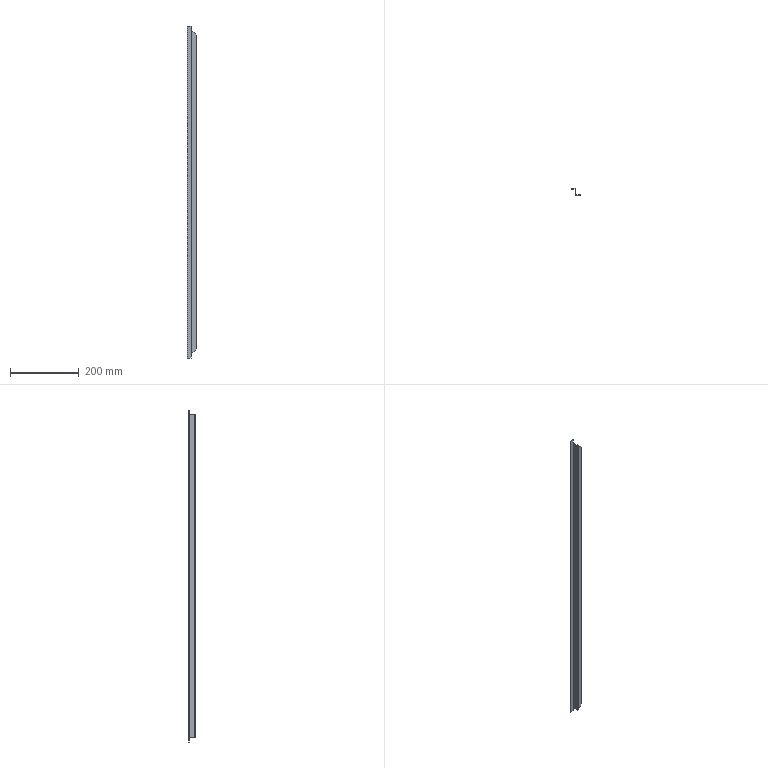Part | STEP file | Left Side Panel Frame Upper | 1 solid | 28 faces | box 26.5 x 20 x 964 mm | volume 62237 mm3 | plane 22 | cylinder 6 | commonest cylinder face diameters 0.15 x2 0.2 x1 1 x1 3.2 x1 4 x1
STEP:
#1=CARTESIAN_POINT('',(0.,-25.93,127.648));
#2=VERTEX_POINT('',#1);
#3=CARTESIAN_POINT('',(0.,-28.08,127.648));
#4=VERTEX_POINT('',#3);
#5=CARTESIAN_POINT('',(0.,0.,127.648));
#6=DIRECTION('',(0.,-1.,0.));
#7=VECTOR('',#6,1000.);
#8=LINE('',#5,#7);
#9=EDGE_CURVE('',#2,#4,#8,.T.);
#10=ORIENTED_EDGE('',*,*,#9,.T.);
#11=CARTESIAN_POINT('',(0.,-28.08,127.598));
#12=VERTEX_POINT('',#11);
#13=CARTESIAN_POINT('',(0.,-28.08,1067.598));
#14=DIRECTION('',(0.,0.,1.));
#15=VECTOR('',#14,1000.);
#16=LINE('',#13,#15);
#17=EDGE_CURVE('',#12,#4,#16,.T.);
#18=ORIENTED_EDGE('',*,*,#17,.F.);
#19=CARTESIAN_POINT('',(0.,-9.68,127.598));
#20=VERTEX_POINT('',#19);
#21=CARTESIAN_POINT('',(0.,0.,127.598));
#22=DIRECTION('',(0.,1.,0.));
#23=VECTOR('',#22,1000.);
#24=LINE('',#21,#23);
#25=EDGE_CURVE('',#12,#20,#24,.T.);
#26=ORIENTED_EDGE('',*,*,#25,.T.);
#27=CARTESIAN_POINT('',(0.,-9.68,1067.598));
#28=VERTEX_POINT('',#27);
#29=CARTESIAN_POINT('',(0.,-9.68,0.));
#30=DIRECTION('',(0.,0.,1.));
#31=VECTOR('',#30,1000.);
#32=LINE('',#29,#31);
#33=EDGE_CURVE('',#20,#28,#32,.T.);
#34=ORIENTED_EDGE('',*,*,#33,.T.);
#35=CARTESIAN_POINT('',(0.,-28.08,1067.598));
#36=VERTEX_POINT('',#35);
#37=CARTESIAN_POINT('',(0.,0.,1067.598));
#38=DIRECTION('',(0.,-1.,0.));
#39=VECTOR('',#38,1000.);
#40=LINE('',#37,#39);
#41=EDGE_CURVE('',#28,#36,#40,.T.);
#42=ORIENTED_EDGE('',*,*,#41,.T.);
#43=CARTESIAN_POINT('',(0.,-28.08,1067.548));
#44=VERTEX_POINT('',#43);
#45=CARTESIAN_POINT('',(0.,-28.08,1067.598));
#46=DIRECTION('',(0.,0.,1.));
#47=VECTOR('',#46,1000.);
#48=LINE('',#45,#47);
#49=EDGE_CURVE('',#44,#36,#48,.T.);
#50=ORIENTED_EDGE('',*,*,#49,.F.);
#51=CARTESIAN_POINT('',(0.,-25.93,1067.548));
#52=VERTEX_POINT('',#51);
#53=CARTESIAN_POINT('',(0.,0.,1067.548));
#54=DIRECTION('',(0.,1.,0.));
#55=VECTOR('',#54,1000.);
#56=LINE('',#53,#55);
#57=EDGE_CURVE('',#44,#52,#56,.T.);
#58=ORIENTED_EDGE('',*,*,#57,.T.);
#59=CARTESIAN_POINT('',(0.,-25.93,1067.398));
#60=VERTEX_POINT('',#59);
#61=CARTESIAN_POINT('',(0.,-25.93,1067.473));
#62=DIRECTION('',(-1.,0.,0.));
#63=DIRECTION('',(0.,0.,1.));
#64=AXIS2_PLACEMENT_3D('',#61,#62,#63);
#65=CIRCLE('',#64,0.075);
#66=EDGE_CURVE('',#52,#60,#65,.T.);
#67=ORIENTED_EDGE('',*,*,#66,.T.);
#68=CARTESIAN_POINT('',(0.,-26.08,1067.398));
#69=VERTEX_POINT('',#68);
#70=CARTESIAN_POINT('',(0.,-26.08,1067.398));
#71=DIRECTION('',(0.,1.,0.));
#72=VECTOR('',#71,1000.);
#73=LINE('',#70,#72);
#74=EDGE_CURVE('',#69,#60,#73,.T.);
#75=ORIENTED_EDGE('',*,*,#74,.F.);
#76=CARTESIAN_POINT('',(0.,-26.08,127.798));
#77=VERTEX_POINT('',#76);
#78=CARTESIAN_POINT('',(0.,-26.08,0.));
#79=DIRECTION('',(0.,0.,-1.));
#80=VECTOR('',#79,1000.);
#81=LINE('',#78,#80);
#82=EDGE_CURVE('',#69,#77,#81,.T.);
#83=ORIENTED_EDGE('',*,*,#82,.T.);
#84=CARTESIAN_POINT('',(0.,-25.93,127.798));
#85=VERTEX_POINT('',#84);
#86=CARTESIAN_POINT('',(0.,-25.93,127.798));
#87=DIRECTION('',(0.,-1.,0.));
#88=VECTOR('',#87,1000.);
#89=LINE('',#86,#88);
#90=EDGE_CURVE('',#85,#77,#89,.T.);
#91=ORIENTED_EDGE('',*,*,#90,.F.);
#92=CARTESIAN_POINT('',(0.,-25.93,127.723));
#93=DIRECTION('',(-1.,0.,0.));
#94=DIRECTION('',(0.,0.,1.));
#95=AXIS2_PLACEMENT_3D('',#92,#93,#94);
#96=CIRCLE('',#95,0.075);
#97=EDGE_CURVE('',#85,#2,#96,.T.);
#98=ORIENTED_EDGE('',*,*,#97,.T.);
#99=EDGE_LOOP('',(#10,#18,#26,#34,#42,#50,#58,#67,#75,#83,#91,#98));
#100=FACE_OUTER_BOUND('',#99,.T.);
#101=CARTESIAN_POINT('',(0.,0.,0.));
#102=DIRECTION('',(1.,0.,0.));
#103=DIRECTION('',(0.,0.,-1.));
#104=AXIS2_PLACEMENT_3D('',#101,#102,#103);
#105=PLANE('',#104);
#106=ADVANCED_FACE('',(#100),#105,.T.);
#107=CARTESIAN_POINT('',(-1.5,-28.08,127.648));
#108=VERTEX_POINT('',#107);
#109=CARTESIAN_POINT('',(0.,-28.08,127.648));
#110=DIRECTION('',(1.,0.,0.));
#111=VECTOR('',#110,1000.);
#112=LINE('',#109,#111);
#113=EDGE_CURVE('',#108,#4,#112,.T.);
#114=ORIENTED_EDGE('',*,*,#113,.T.);
#115=ORIENTED_EDGE('',*,*,#9,.F.);
#116=CARTESIAN_POINT('',(-1.5,-25.93,127.648));
#117=VERTEX_POINT('',#116);
#118=CARTESIAN_POINT('',(0.,-25.93,127.648));
#119=DIRECTION('',(-1.,0.,0.));
#120=VECTOR('',#119,1000.);
#121=LINE('',#118,#120);
#122=EDGE_CURVE('',#2,#117,#121,.T.);
#123=ORIENTED_EDGE('',*,*,#122,.T.);
#124=CARTESIAN_POINT('',(-1.5,-28.08,127.648));
#125=DIRECTION('',(0.,-1.,0.));
#126=VECTOR('',#125,1000.);
#127=LINE('',#124,#126);
#128=EDGE_CURVE('',#117,#108,#127,.T.);
#129=ORIENTED_EDGE('',*,*,#128,.T.);
#130=EDGE_LOOP('',(#114,#115,#123,#129));
#131=FACE_OUTER_BOUND('',#130,.T.);
#132=CARTESIAN_POINT('',(0.,-28.08,127.648));
#133=DIRECTION('',(0.,0.,1.));
#134=DIRECTION('',(0.,-1.,0.));
#135=AXIS2_PLACEMENT_3D('',#132,#133,#134);
#136=PLANE('',#135);
#137=ADVANCED_FACE('',(#131),#136,.T.);
#138=CARTESIAN_POINT('',(0.5,-26.58,1067.098));
#139=VERTEX_POINT('',#138);
#140=CARTESIAN_POINT('',(0.2,-26.48,1067.398));
#141=VERTEX_POINT('',#140);
#142=CARTESIAN_POINT('',(0.5,-26.58,1067.098));
#143=CARTESIAN_POINT('',(0.3909,-26.58,1067.207));
#144=CARTESIAN_POINT('',(0.2873,-26.546,1067.311));
#145=CARTESIAN_POINT('',(0.2,-26.48,1067.398));
#146=(BOUNDED_CURVE()B_SPLINE_CURVE(3,(#142,#143,#144,#145),.UNSPECIFIED.,.F.,.F.)B_SPLINE_CURVE_WITH_KNOTS((4,4),(1.571,2.214),.UNSPECIFIED.)CURVE()GEOMETRIC_REPRESENTATION_ITEM()RATIONAL_B_SPLINE_CURVE((1.,0.9658,0.9658,1.))REPRESENTATION_ITEM(''));
#147=EDGE_CURVE('',#139,#141,#146,.T.);
#148=ORIENTED_EDGE('',*,*,#147,.F.);
#149=CARTESIAN_POINT('',(0.5,-26.58,128.098));
#150=VERTEX_POINT('',#149);
#151=CARTESIAN_POINT('',(0.5,-26.58,127.798));
#152=DIRECTION('',(0.,0.,1.));
#153=VECTOR('',#152,1000.);
#154=LINE('',#151,#153);
#155=EDGE_CURVE('',#150,#139,#154,.T.);
#156=ORIENTED_EDGE('',*,*,#155,.F.);
#157=CARTESIAN_POINT('',(0.2,-26.48,127.798));
#158=VERTEX_POINT('',#157);
#159=CARTESIAN_POINT('',(0.5,-26.58,128.098));
#160=CARTESIAN_POINT('',(0.3909,-26.58,127.989));
#161=CARTESIAN_POINT('',(0.2873,-26.546,127.885));
#162=CARTESIAN_POINT('',(0.2,-26.48,127.798));
#163=(BOUNDED_CURVE()B_SPLINE_CURVE(3,(#159,#160,#161,#162),.UNSPECIFIED.,.F.,.F.)B_SPLINE_CURVE_WITH_KNOTS((4,4),(4.712,5.356),.UNSPECIFIED.)CURVE()GEOMETRIC_REPRESENTATION_ITEM()RATIONAL_B_SPLINE_CURVE((1.,0.9658,0.9658,1.))REPRESENTATION_ITEM(''));
#164=EDGE_CURVE('',#150,#158,#163,.T.);
#165=ORIENTED_EDGE('',*,*,#164,.T.);
#166=CARTESIAN_POINT('',(0.5,-26.08,127.798));
#167=DIRECTION('',(0.,0.,-1.));
#168=DIRECTION('',(-1.,0.,0.));
#169=AXIS2_PLACEMENT_3D('',#166,#167,#168);
#170=CIRCLE('',#169,0.5);
#171=EDGE_CURVE('',#158,#77,#170,.T.);
#172=ORIENTED_EDGE('',*,*,#171,.T.);
#173=ORIENTED_EDGE('',*,*,#82,.F.);
#174=CARTESIAN_POINT('',(0.5,-26.08,1067.398));
#175=DIRECTION('',(0.,0.,-1.));
#176=DIRECTION('',(-1.,0.,0.));
#177=AXIS2_PLACEMENT_3D('',#174,#175,#176);
#178=CIRCLE('',#177,0.5);
#179=EDGE_CURVE('',#141,#69,#178,.T.);
#180=ORIENTED_EDGE('',*,*,#179,.F.);
#181=EDGE_LOOP('',(#148,#156,#165,#172,#173,#180));
#182=FACE_OUTER_BOUND('',#181,.T.);
#183=CARTESIAN_POINT('',(0.5,-26.08,127.798));
#184=DIRECTION('',(0.,0.,-1.));
#185=DIRECTION('',(-1.,0.,0.));
#186=AXIS2_PLACEMENT_3D('',#183,#184,#185);
#187=CYLINDRICAL_SURFACE('',#186,0.5);
#188=ADVANCED_FACE('',(#182),#187,.F.);
#189=CARTESIAN_POINT('',(-1.5,-25.93,1067.548));
#190=VERTEX_POINT('',#189);
#191=CARTESIAN_POINT('',(0.,-25.93,1067.548));
#192=DIRECTION('',(1.,0.,0.));
#193=VECTOR('',#192,1000.);
#194=LINE('',#191,#193);
#195=EDGE_CURVE('',#190,#52,#194,.T.);
#196=ORIENTED_EDGE('',*,*,#195,.T.);
#197=ORIENTED_EDGE('',*,*,#57,.F.);
#198=CARTESIAN_POINT('',(-1.5,-28.08,1067.548));
#199=VERTEX_POINT('',#198);
#200=CARTESIAN_POINT('',(0.,-28.08,1067.548));
#201=DIRECTION('',(-1.,0.,0.));
#202=VECTOR('',#201,1000.);
#203=LINE('',#200,#202);
#204=EDGE_CURVE('',#44,#199,#203,.T.);
#205=ORIENTED_EDGE('',*,*,#204,.T.);
#206=CARTESIAN_POINT('',(-1.5,-25.93,1067.548));
#207=DIRECTION('',(0.,1.,0.));
#208=VECTOR('',#207,1000.);
#209=LINE('',#206,#208);
#210=EDGE_CURVE('',#199,#190,#209,.T.);
#211=ORIENTED_EDGE('',*,*,#210,.T.);
#212=EDGE_LOOP('',(#196,#197,#205,#211));
#213=FACE_OUTER_BOUND('',#212,.T.);
#214=CARTESIAN_POINT('',(0.,-25.93,1067.548));
#215=DIRECTION('',(0.,0.,-1.));
#216=DIRECTION('',(-1.,0.,0.));
#217=AXIS2_PLACEMENT_3D('',#214,#215,#216);
#218=PLANE('',#217);
#219=ADVANCED_FACE('',(#213),#218,.T.);
#220=CARTESIAN_POINT('',(-1.5,-28.08,1067.598));
#221=VERTEX_POINT('',#220);
#222=CARTESIAN_POINT('',(-1.5,-28.08,1067.598));
#223=DIRECTION('',(1.,0.,0.));
#224=VECTOR('',#223,1000.);
#225=LINE('',#222,#224);
#226=EDGE_CURVE('',#221,#36,#225,.T.);
#227=ORIENTED_EDGE('',*,*,#226,.T.);
#228=ORIENTED_EDGE('',*,*,#41,.F.);
#229=CARTESIAN_POINT('',(-1.6,-8.08,1067.598));
#230=VERTEX_POINT('',#229);
#231=CARTESIAN_POINT('',(-1.6,-9.68,1067.598));
#232=DIRECTION('',(0.,0.,-1.));
#233=DIRECTION('',(-1.,0.,0.));
#234=AXIS2_PLACEMENT_3D('',#231,#232,#233);
#235=CIRCLE('',#234,1.6);
#236=EDGE_CURVE('',#230,#28,#235,.T.);
#237=ORIENTED_EDGE('',*,*,#236,.F.);
#238=CARTESIAN_POINT('',(-1.6,-9.58,1067.598));
#239=VERTEX_POINT('',#238);
#240=CARTESIAN_POINT('',(-1.6,-9.58,1067.598));
#241=DIRECTION('',(0.,-1.,0.));
#242=VECTOR('',#241,1000.);
#243=LINE('',#240,#242);
#244=EDGE_CURVE('',#230,#239,#243,.T.);
#245=ORIENTED_EDGE('',*,*,#244,.T.);
#246=CARTESIAN_POINT('',(-1.5,-9.68,1067.598));
#247=VERTEX_POINT('',#246);
#248=CARTESIAN_POINT('',(-1.6,-9.68,1067.598));
#249=DIRECTION('',(0.,0.,-1.));
#250=DIRECTION('',(-1.,0.,0.));
#251=AXIS2_PLACEMENT_3D('',#248,#249,#250);
#252=CIRCLE('',#251,0.1);
#253=EDGE_CURVE('',#239,#247,#252,.T.);
#254=ORIENTED_EDGE('',*,*,#253,.T.);
#255=CARTESIAN_POINT('',(-1.5,-8.08,1067.598));
#256=DIRECTION('',(0.,-1.,0.));
#257=VECTOR('',#256,1000.);
#258=LINE('',#255,#257);
#259=EDGE_CURVE('',#247,#221,#258,.T.);
#260=ORIENTED_EDGE('',*,*,#259,.T.);
#261=EDGE_LOOP('',(#227,#228,#237,#245,#254,#260));
#262=FACE_OUTER_BOUND('',#261,.T.);
#263=CARTESIAN_POINT('',(-1.5,-8.08,1067.598));
#264=DIRECTION('',(0.,0.,1.));
#265=DIRECTION('',(1.,0.,0.));
#266=AXIS2_PLACEMENT_3D('',#263,#264,#265);
#267=PLANE('',#266);
#268=ADVANCED_FACE('',(#262),#267,.T.);
#269=CARTESIAN_POINT('',(-1.6,-8.08,127.598));
#270=VERTEX_POINT('',#269);
#271=CARTESIAN_POINT('',(-1.6,-8.08,127.598));
#272=DIRECTION('',(0.,0.,1.));
#273=VECTOR('',#272,1000.);
#274=LINE('',#271,#273);
#275=EDGE_CURVE('',#270,#230,#274,.T.);
#276=ORIENTED_EDGE('',*,*,#275,.T.);
#277=ORIENTED_EDGE('',*,*,#236,.T.);
#278=ORIENTED_EDGE('',*,*,#33,.F.);
#279=CARTESIAN_POINT('',(-1.6,-9.68,127.598));
#280=DIRECTION('',(0.,0.,1.));
#281=DIRECTION('',(-1.,0.,0.));
#282=AXIS2_PLACEMENT_3D('',#279,#280,#281);
#283=CIRCLE('',#282,1.6);
#284=EDGE_CURVE('',#20,#270,#283,.T.);
#285=ORIENTED_EDGE('',*,*,#284,.T.);
#286=EDGE_LOOP('',(#276,#277,#278,#285));
#287=FACE_OUTER_BOUND('',#286,.T.);
#288=CARTESIAN_POINT('',(-1.6,-9.68,127.598));
#289=DIRECTION('',(0.,0.,-1.));
#290=DIRECTION('',(-1.,0.,0.));
#291=AXIS2_PLACEMENT_3D('',#288,#289,#290);
#292=CYLINDRICAL_SURFACE('',#291,1.6);
#293=ADVANCED_FACE('',(#287),#292,.T.);
#294=ORIENTED_EDGE('',*,*,#25,.F.);
#295=CARTESIAN_POINT('',(-1.5,-28.08,127.598));
#296=VERTEX_POINT('',#295);
#297=CARTESIAN_POINT('',(-1.5,-28.08,127.598));
#298=DIRECTION('',(-1.,0.,0.));
#299=VECTOR('',#298,1000.);
#300=LINE('',#297,#299);
#301=EDGE_CURVE('',#12,#296,#300,.T.);
#302=ORIENTED_EDGE('',*,*,#301,.T.);
#303=CARTESIAN_POINT('',(-1.5,-9.68,127.598));
#304=VERTEX_POINT('',#303);
#305=CARTESIAN_POINT('',(-1.5,-28.08,127.598));
#306=DIRECTION('',(0.,1.,0.));
#307=VECTOR('',#306,1000.);
#308=LINE('',#305,#307);
#309=EDGE_CURVE('',#296,#304,#308,.T.);
#310=ORIENTED_EDGE('',*,*,#309,.T.);
#311=CARTESIAN_POINT('',(-1.6,-9.58,127.598));
#312=VERTEX_POINT('',#311);
#313=CARTESIAN_POINT('',(-1.6,-9.68,127.598));
#314=DIRECTION('',(0.,0.,-1.));
#315=DIRECTION('',(-1.,0.,0.));
#316=AXIS2_PLACEMENT_3D('',#313,#314,#315);
#317=CIRCLE('',#316,0.1);
#318=EDGE_CURVE('',#312,#304,#317,.T.);
#319=ORIENTED_EDGE('',*,*,#318,.F.);
#320=CARTESIAN_POINT('',(-1.6,-9.68,127.598));
#321=DIRECTION('',(0.,-1.,0.));
#322=VECTOR('',#321,1000.);
#323=LINE('',#320,#322);
#324=EDGE_CURVE('',#270,#312,#323,.T.);
#325=ORIENTED_EDGE('',*,*,#324,.F.);
#326=ORIENTED_EDGE('',*,*,#284,.F.);
#327=EDGE_LOOP('',(#294,#302,#310,#319,#325,#326));
#328=FACE_OUTER_BOUND('',#327,.T.);
#329=CARTESIAN_POINT('',(-1.5,-28.08,127.598));
#330=DIRECTION('',(0.,0.,-1.));
#331=DIRECTION('',(-1.,0.,0.));
#332=AXIS2_PLACEMENT_3D('',#329,#330,#331);
#333=PLANE('',#332);
#334=ADVANCED_FACE('',(#328),#333,.T.);
#335=CARTESIAN_POINT('',(-1.5,-28.08,1067.598));
#336=DIRECTION('',(0.,0.,-1.));
#337=VECTOR('',#336,1000.);
#338=LINE('',#335,#337);
#339=EDGE_CURVE('',#108,#296,#338,.T.);
#340=ORIENTED_EDGE('',*,*,#339,.T.);
#341=ORIENTED_EDGE('',*,*,#301,.F.);
#342=ORIENTED_EDGE('',*,*,#17,.T.);
#343=ORIENTED_EDGE('',*,*,#113,.F.);
#344=EDGE_LOOP('',(#340,#341,#342,#343));
#345=FACE_OUTER_BOUND('',#344,.T.);
#346=CARTESIAN_POINT('',(-1.5,-28.08,1067.598));
#347=DIRECTION('',(0.,-1.,0.));
#348=DIRECTION('',(0.,0.,-1.));
#349=AXIS2_PLACEMENT_3D('',#346,#347,#348);
#350=PLANE('',#349);
#351=ADVANCED_FACE('',(#345),#350,.T.);
#352=ORIENTED_EDGE('',*,*,#309,.F.);
#353=ORIENTED_EDGE('',*,*,#339,.F.);
#354=ORIENTED_EDGE('',*,*,#128,.F.);
#355=CARTESIAN_POINT('',(-1.5,-25.93,127.798));
#356=VERTEX_POINT('',#355);
#357=CARTESIAN_POINT('',(-1.5,-25.93,127.723));
#358=DIRECTION('',(-1.,0.,0.));
#359=DIRECTION('',(0.,0.,1.));
#360=AXIS2_PLACEMENT_3D('',#357,#358,#359);
#361=CIRCLE('',#360,0.075);
#362=EDGE_CURVE('',#356,#117,#361,.T.);
#363=ORIENTED_EDGE('',*,*,#362,.F.);
#364=CARTESIAN_POINT('',(-1.5,-26.08,127.798));
#365=VERTEX_POINT('',#364);
#366=CARTESIAN_POINT('',(-1.5,-25.93,127.798));
#367=DIRECTION('',(0.,1.,0.));
#368=VECTOR('',#367,1000.);
#369=LINE('',#366,#368);
#370=EDGE_CURVE('',#365,#356,#369,.T.);
#371=ORIENTED_EDGE('',*,*,#370,.F.);
#372=CARTESIAN_POINT('',(-1.5,-26.08,1067.398));
#373=VERTEX_POINT('',#372);
#374=CARTESIAN_POINT('',(-1.5,-26.08,0.));
#375=DIRECTION('',(0.,0.,-1.));
#376=VECTOR('',#375,1000.);
#377=LINE('',#374,#376);
#378=EDGE_CURVE('',#373,#365,#377,.T.);
#379=ORIENTED_EDGE('',*,*,#378,.F.);
#380=CARTESIAN_POINT('',(-1.5,-25.93,1067.398));
#381=VERTEX_POINT('',#380);
#382=CARTESIAN_POINT('',(-1.5,-26.08,1067.398));
#383=DIRECTION('',(0.,-1.,0.));
#384=VECTOR('',#383,1000.);
#385=LINE('',#382,#384);
#386=EDGE_CURVE('',#381,#373,#385,.T.);
#387=ORIENTED_EDGE('',*,*,#386,.F.);
#388=CARTESIAN_POINT('',(-1.5,-25.93,1067.473));
#389=DIRECTION('',(-1.,0.,0.));
#390=DIRECTION('',(0.,0.,1.));
#391=AXIS2_PLACEMENT_3D('',#388,#389,#390);
#392=CIRCLE('',#391,0.075);
#393=EDGE_CURVE('',#190,#381,#392,.T.);
#394=ORIENTED_EDGE('',*,*,#393,.F.);
#395=ORIENTED_EDGE('',*,*,#210,.F.);
#396=CARTESIAN_POINT('',(-1.5,-28.08,0.));
#397=DIRECTION('',(0.,0.,-1.));
#398=VECTOR('',#397,1000.);
#399=LINE('',#396,#398);
#400=EDGE_CURVE('',#221,#199,#399,.T.);
#401=ORIENTED_EDGE('',*,*,#400,.F.);
#402=ORIENTED_EDGE('',*,*,#259,.F.);
#403=CARTESIAN_POINT('',(-1.5,-9.68,0.));
#404=DIRECTION('',(0.,0.,1.));
#405=VECTOR('',#404,1000.);
#406=LINE('',#403,#405);
#407=EDGE_CURVE('',#304,#247,#406,.T.);
#408=ORIENTED_EDGE('',*,*,#407,.F.);
#409=EDGE_LOOP('',(#352,#353,#354,#363,#371,#379,#387,#394,#395,#401,#402,#408));
#410=FACE_OUTER_BOUND('',#409,.T.);
#411=CARTESIAN_POINT('',(-1.5,0.,0.));
#412=DIRECTION('',(1.,0.,0.));
#413=DIRECTION('',(0.,0.,-1.));
#414=AXIS2_PLACEMENT_3D('',#411,#412,#413);
#415=PLANE('',#414);
#416=ADVANCED_FACE('',(#410),#415,.F.);
#417=ORIENTED_EDGE('',*,*,#362,.T.);
#418=ORIENTED_EDGE('',*,*,#122,.F.);
#419=ORIENTED_EDGE('',*,*,#97,.F.);
#420=CARTESIAN_POINT('',(0.,-25.93,127.798));
#421=DIRECTION('',(1.,0.,0.));
#422=VECTOR('',#421,1000.);
#423=LINE('',#420,#422);
#424=EDGE_CURVE('',#356,#85,#423,.T.);
#425=ORIENTED_EDGE('',*,*,#424,.F.);
#426=EDGE_LOOP('',(#417,#418,#419,#425));
#427=FACE_OUTER_BOUND('',#426,.T.);
#428=CARTESIAN_POINT('',(0.,-25.93,127.723));
#429=DIRECTION('',(-1.,0.,0.));
#430=DIRECTION('',(0.,0.,1.));
#431=AXIS2_PLACEMENT_3D('',#428,#429,#430);
#432=CYLINDRICAL_SURFACE('',#431,0.075);
#433=ADVANCED_FACE('',(#427),#432,.F.);
#434=CARTESIAN_POINT('',(14.5,-26.58,1053.098));
#435=VERTEX_POINT('',#434);
#436=CARTESIAN_POINT('',(14.5,-26.58,142.098));
#437=VERTEX_POINT('',#436);
#438=CARTESIAN_POINT('',(14.5,-26.58,0.));
#439=DIRECTION('',(0.,0.,-1.));
#440=VECTOR('',#439,1000.);
#441=LINE('',#438,#440);
#442=EDGE_CURVE('',#435,#437,#441,.T.);
#443=ORIENTED_EDGE('',*,*,#442,.T.);
#444=CARTESIAN_POINT('',(14.5,-26.58,142.098));
#445=DIRECTION('',(-0.7071,0.,-0.7071));
#446=VECTOR('',#445,1000.);
#447=LINE('',#444,#446);
#448=EDGE_CURVE('',#437,#150,#447,.T.);
#449=ORIENTED_EDGE('',*,*,#448,.T.);
#450=ORIENTED_EDGE('',*,*,#155,.T.);
#451=CARTESIAN_POINT('',(0.5,-26.58,1067.098));
#452=DIRECTION('',(0.7071,0.,-0.7071));
#453=VECTOR('',#452,1000.);
#454=LINE('',#451,#453);
#455=EDGE_CURVE('',#139,#435,#454,.T.);
#456=ORIENTED_EDGE('',*,*,#455,.T.);
#457=EDGE_LOOP('',(#443,#449,#450,#456));
#458=FACE_OUTER_BOUND('',#457,.T.);
#459=CARTESIAN_POINT('',(0.,-26.58,0.));
#460=DIRECTION('',(0.,1.,0.));
#461=DIRECTION('',(-1.,0.,0.));
#462=AXIS2_PLACEMENT_3D('',#459,#460,#461);
#463=PLANE('',#462);
#464=ADVANCED_FACE('',(#458),#463,.T.);
#465=ORIENTED_EDGE('',*,*,#393,.T.);
#466=CARTESIAN_POINT('',(0.,-25.93,1067.398));
#467=DIRECTION('',(-1.,0.,0.));
#468=VECTOR('',#467,1000.);
#469=LINE('',#466,#468);
#470=EDGE_CURVE('',#60,#381,#469,.T.);
#471=ORIENTED_EDGE('',*,*,#470,.F.);
#472=ORIENTED_EDGE('',*,*,#66,.F.);
#473=ORIENTED_EDGE('',*,*,#195,.F.);
#474=EDGE_LOOP('',(#465,#471,#472,#473));
#475=FACE_OUTER_BOUND('',#474,.T.);
#476=CARTESIAN_POINT('',(0.,-25.93,1067.473));
#477=DIRECTION('',(-1.,0.,0.));
#478=DIRECTION('',(0.,0.,1.));
#479=AXIS2_PLACEMENT_3D('',#476,#477,#478);
#480=CYLINDRICAL_SURFACE('',#479,0.075);
#481=ADVANCED_FACE('',(#475),#480,.F.);
#482=ORIENTED_EDGE('',*,*,#49,.T.);
#483=ORIENTED_EDGE('',*,*,#226,.F.);
#484=ORIENTED_EDGE('',*,*,#400,.T.);
#485=ORIENTED_EDGE('',*,*,#204,.F.);
#486=EDGE_LOOP('',(#482,#483,#484,#485));
#487=FACE_OUTER_BOUND('',#486,.T.);
#488=CARTESIAN_POINT('',(-1.5,-28.08,1067.598));
#489=DIRECTION('',(0.,-1.,0.));
#490=DIRECTION('',(0.,0.,-1.));
#491=AXIS2_PLACEMENT_3D('',#488,#489,#490);
#492=PLANE('',#491);
#493=ADVANCED_FACE('',(#487),#492,.T.);
#494=CARTESIAN_POINT('',(-1.6,-8.08,115.598));
#495=VERTEX_POINT('',#494);
#496=CARTESIAN_POINT('',(-1.6,-8.08,0.));
#497=DIRECTION('',(0.,0.,-1.));
#498=VECTOR('',#497,1000.);
#499=LINE('',#496,#498);
#500=EDGE_CURVE('',#270,#495,#499,.T.);
#501=ORIENTED_EDGE('',*,*,#500,.T.);
#502=CARTESIAN_POINT('',(-12.,-8.08,115.598));
#503=VERTEX_POINT('',#502);
#504=CARTESIAN_POINT('',(0.,-8.08,115.598));
#505=DIRECTION('',(-1.,0.,0.));
#506=VECTOR('',#505,1000.);
#507=LINE('',#504,#506);
#508=EDGE_CURVE('',#495,#503,#507,.T.);
#509=ORIENTED_EDGE('',*,*,#508,.T.);
#510=CARTESIAN_POINT('',(-12.,-8.08,1079.598));
#511=VERTEX_POINT('',#510);
#512=CARTESIAN_POINT('',(-12.,-8.08,0.));
#513=DIRECTION('',(0.,0.,1.));
#514=VECTOR('',#513,1000.);
#515=LINE('',#512,#514);
#516=EDGE_CURVE('',#503,#511,#515,.T.);
#517=ORIENTED_EDGE('',*,*,#516,.T.);
#518=CARTESIAN_POINT('',(-1.6,-8.08,1079.598));
#519=VERTEX_POINT('',#518);
#520=CARTESIAN_POINT('',(0.,-8.08,1079.598));
#521=DIRECTION('',(1.,0.,0.));
#522=VECTOR('',#521,1000.);
#523=LINE('',#520,#522);
#524=EDGE_CURVE('',#511,#519,#523,.T.);
#525=ORIENTED_EDGE('',*,*,#524,.T.);
#526=CARTESIAN_POINT('',(-1.6,-8.08,0.));
#527=DIRECTION('',(0.,0.,-1.));
#528=VECTOR('',#527,1000.);
#529=LINE('',#526,#528);
#530=EDGE_CURVE('',#519,#230,#529,.T.);
#531=ORIENTED_EDGE('',*,*,#530,.T.);
#532=ORIENTED_EDGE('',*,*,#275,.F.);
#533=EDGE_LOOP('',(#501,#509,#517,#525,#531,#532));
#534=FACE_OUTER_BOUND('',#533,.T.);
#535=CARTESIAN_POINT('',(0.,-8.08,0.));
#536=DIRECTION('',(0.,1.,0.));
#537=DIRECTION('',(-1.,0.,0.));
#538=AXIS2_PLACEMENT_3D('',#535,#536,#537);
#539=PLANE('',#538);
#540=ADVANCED_FACE('',(#534),#539,.T.);
#541=ORIENTED_EDGE('',*,*,#253,.F.);
#542=CARTESIAN_POINT('',(-1.6,-9.58,127.598));
#543=DIRECTION('',(0.,0.,1.));
#544=VECTOR('',#543,1000.);
#545=LINE('',#542,#544);
#546=EDGE_CURVE('',#312,#239,#545,.T.);
#547=ORIENTED_EDGE('',*,*,#546,.F.);
#548=ORIENTED_EDGE('',*,*,#318,.T.);
#549=ORIENTED_EDGE('',*,*,#407,.T.);
#550=EDGE_LOOP('',(#541,#547,#548,#549));
#551=FACE_OUTER_BOUND('',#550,.T.);
#552=CARTESIAN_POINT('',(-1.6,-9.68,127.598));
#553=DIRECTION('',(0.,0.,-1.));
#554=DIRECTION('',(-1.,0.,0.));
#555=AXIS2_PLACEMENT_3D('',#552,#553,#554);
#556=CYLINDRICAL_SURFACE('',#555,0.1);
#557=ADVANCED_FACE('',(#551),#556,.F.);
#558=CARTESIAN_POINT('',(0.2,-28.057,127.798));
#559=VERTEX_POINT('',#558);
#560=CARTESIAN_POINT('',(0.5,-26.08,127.798));
#561=DIRECTION('',(0.,0.,1.));
#562=DIRECTION('',(-1.,0.,0.));
#563=AXIS2_PLACEMENT_3D('',#560,#561,#562);
#564=CIRCLE('',#563,2.);
#565=EDGE_CURVE('',#365,#559,#564,.T.);
#566=ORIENTED_EDGE('',*,*,#565,.T.);
#567=CARTESIAN_POINT('',(0.5,-28.08,128.098));
#568=VERTEX_POINT('',#567);
#569=CARTESIAN_POINT('',(0.2,-28.057,127.798));
#570=CARTESIAN_POINT('',(0.2993,-28.072,127.897));
#571=CARTESIAN_POINT('',(0.3995,-28.08,127.997));
#572=CARTESIAN_POINT('',(0.5,-28.08,128.098));
#573=(BOUNDED_CURVE()B_SPLINE_CURVE(3,(#569,#570,#571,#572),.UNSPECIFIED.,.F.,.F.)B_SPLINE_CURVE_WITH_KNOTS((4,4),(1.42,1.571),.UNSPECIFIED.)CURVE()GEOMETRIC_REPRESENTATION_ITEM()RATIONAL_B_SPLINE_CURVE((1.,0.9981,0.9981,1.))REPRESENTATION_ITEM(''));
#574=EDGE_CURVE('',#559,#568,#573,.T.);
#575=ORIENTED_EDGE('',*,*,#574,.T.);
#576=CARTESIAN_POINT('',(0.5,-28.08,1067.098));
#577=VERTEX_POINT('',#576);
#578=CARTESIAN_POINT('',(0.5,-28.08,127.798));
#579=DIRECTION('',(0.,0.,1.));
#580=VECTOR('',#579,1000.);
#581=LINE('',#578,#580);
#582=EDGE_CURVE('',#568,#577,#581,.T.);
#583=ORIENTED_EDGE('',*,*,#582,.T.);
#584=CARTESIAN_POINT('',(0.2,-28.057,1067.398));
#585=VERTEX_POINT('',#584);
#586=CARTESIAN_POINT('',(0.5,-28.08,1067.098));
#587=CARTESIAN_POINT('',(0.3995,-28.08,1067.198));
#588=CARTESIAN_POINT('',(0.2993,-28.072,1067.299));
#589=CARTESIAN_POINT('',(0.2,-28.057,1067.398));
#590=(BOUNDED_CURVE()B_SPLINE_CURVE(3,(#586,#587,#588,#589),.UNSPECIFIED.,.F.,.F.)B_SPLINE_CURVE_WITH_KNOTS((4,4),(1.571,1.721),.UNSPECIFIED.)CURVE()GEOMETRIC_REPRESENTATION_ITEM()RATIONAL_B_SPLINE_CURVE((1.,0.9981,0.9981,1.))REPRESENTATION_ITEM(''));
#591=EDGE_CURVE('',#577,#585,#590,.T.);
#592=ORIENTED_EDGE('',*,*,#591,.T.);
#593=CARTESIAN_POINT('',(0.5,-26.08,1067.398));
#594=DIRECTION('',(0.,0.,-1.));
#595=DIRECTION('',(-1.,0.,0.));
#596=AXIS2_PLACEMENT_3D('',#593,#594,#595);
#597=CIRCLE('',#596,2.);
#598=EDGE_CURVE('',#585,#373,#597,.T.);
#599=ORIENTED_EDGE('',*,*,#598,.T.);
#600=ORIENTED_EDGE('',*,*,#378,.T.);
#601=EDGE_LOOP('',(#566,#575,#583,#592,#599,#600));
#602=FACE_OUTER_BOUND('',#601,.T.);
#603=CARTESIAN_POINT('',(0.5,-26.08,127.798));
#604=DIRECTION('',(0.,0.,-1.));
#605=DIRECTION('',(-1.,0.,0.));
#606=AXIS2_PLACEMENT_3D('',#603,#604,#605);
#607=CYLINDRICAL_SURFACE('',#606,2.);
#608=ADVANCED_FACE('',(#602),#607,.T.);
#609=ORIENTED_EDGE('',*,*,#424,.T.);
#610=ORIENTED_EDGE('',*,*,#90,.T.);
#611=ORIENTED_EDGE('',*,*,#171,.F.);
#612=CARTESIAN_POINT('',(0.2,-28.08,127.798));
#613=DIRECTION('',(0.,-1.,0.));
#614=VECTOR('',#613,1000.);
#615=LINE('',#612,#614);
#616=EDGE_CURVE('',#158,#559,#615,.T.);
#617=ORIENTED_EDGE('',*,*,#616,.T.);
#618=ORIENTED_EDGE('',*,*,#565,.F.);
#619=ORIENTED_EDGE('',*,*,#370,.T.);
#620=EDGE_LOOP('',(#609,#610,#611,#617,#618,#619));
#621=FACE_OUTER_BOUND('',#620,.T.);
#622=CARTESIAN_POINT('',(0.,-25.93,127.798));
#623=DIRECTION('',(0.,0.,-1.));
#624=DIRECTION('',(-1.,0.,0.));
#625=AXIS2_PLACEMENT_3D('',#622,#623,#624);
#626=PLANE('',#625);
#627=ADVANCED_FACE('',(#621),#626,.T.);
#628=ORIENTED_EDGE('',*,*,#616,.F.);
#629=ORIENTED_EDGE('',*,*,#164,.F.);
#630=ORIENTED_EDGE('',*,*,#448,.F.);
#631=CARTESIAN_POINT('',(14.5,-28.08,142.098));
#632=VERTEX_POINT('',#631);
#633=CARTESIAN_POINT('',(14.5,-28.08,142.098));
#634=DIRECTION('',(0.,1.,0.));
#635=VECTOR('',#634,1000.);
#636=LINE('',#633,#635);
#637=EDGE_CURVE('',#632,#437,#636,.T.);
#638=ORIENTED_EDGE('',*,*,#637,.F.);
#639=CARTESIAN_POINT('',(14.5,-28.08,142.098));
#640=DIRECTION('',(0.7071,0.,0.7071));
#641=VECTOR('',#640,1000.);
#642=LINE('',#639,#641);
#643=EDGE_CURVE('',#568,#632,#642,.T.);
#644=ORIENTED_EDGE('',*,*,#643,.F.);
#645=ORIENTED_EDGE('',*,*,#574,.F.);
#646=EDGE_LOOP('',(#628,#629,#630,#638,#644,#645));
#647=FACE_OUTER_BOUND('',#646,.T.);
#648=CARTESIAN_POINT('',(14.5,-28.08,142.098));
#649=DIRECTION('',(-0.7071,0.,0.7071));
#650=DIRECTION('',(0.7071,0.,0.7071));
#651=AXIS2_PLACEMENT_3D('',#648,#649,#650);
#652=PLANE('',#651);
#653=ADVANCED_FACE('',(#647),#652,.F.);
#654=CARTESIAN_POINT('',(14.5,-28.08,1053.098));
#655=VERTEX_POINT('',#654);
#656=CARTESIAN_POINT('',(14.5,-28.08,1053.098));
#657=DIRECTION('',(0.,1.,0.));
#658=VECTOR('',#657,1000.);
#659=LINE('',#656,#658);
#660=EDGE_CURVE('',#655,#435,#659,.T.);
#661=ORIENTED_EDGE('',*,*,#660,.F.);
#662=CARTESIAN_POINT('',(14.5,-28.08,1067.398));
#663=DIRECTION('',(0.,0.,1.));
#664=VECTOR('',#663,1000.);
#665=LINE('',#662,#664);
#666=EDGE_CURVE('',#632,#655,#665,.T.);
#667=ORIENTED_EDGE('',*,*,#666,.F.);
#668=ORIENTED_EDGE('',*,*,#637,.T.);
#669=ORIENTED_EDGE('',*,*,#442,.F.);
#670=EDGE_LOOP('',(#661,#667,#668,#669));
#671=FACE_OUTER_BOUND('',#670,.T.);
#672=CARTESIAN_POINT('',(14.5,-28.08,1067.398));
#673=DIRECTION('',(-1.,0.,0.));
#674=DIRECTION('',(0.,-1.,0.));
#675=AXIS2_PLACEMENT_3D('',#672,#673,#674);
#676=PLANE('',#675);
#677=ADVANCED_FACE('',(#671),#676,.F.);
#678=CARTESIAN_POINT('',(0.2,-26.08,1067.398));
#679=DIRECTION('',(0.,-1.,0.));
#680=VECTOR('',#679,1000.);
#681=LINE('',#678,#680);
#682=EDGE_CURVE('',#141,#585,#681,.T.);
#683=ORIENTED_EDGE('',*,*,#682,.T.);
#684=ORIENTED_EDGE('',*,*,#591,.F.);
#685=CARTESIAN_POINT('',(0.2,-28.08,1067.398));
#686=DIRECTION('',(0.7071,0.,-0.7071));
#687=VECTOR('',#686,1000.);
#688=LINE('',#685,#687);
#689=EDGE_CURVE('',#577,#655,#688,.T.);
#690=ORIENTED_EDGE('',*,*,#689,.T.);
#691=ORIENTED_EDGE('',*,*,#660,.T.);
#692=ORIENTED_EDGE('',*,*,#455,.F.);
#693=ORIENTED_EDGE('',*,*,#147,.T.);
#694=EDGE_LOOP('',(#683,#684,#690,#691,#692,#693));
#695=FACE_OUTER_BOUND('',#694,.T.);
#696=CARTESIAN_POINT('',(0.2,-26.08,1067.398));
#697=DIRECTION('',(0.7071,0.,0.7071));
#698=DIRECTION('',(0.7071,0.,-0.7071));
#699=AXIS2_PLACEMENT_3D('',#696,#697,#698);
#700=PLANE('',#699);
#701=ADVANCED_FACE('',(#695),#700,.T.);
#702=ORIENTED_EDGE('',*,*,#386,.T.);
#703=ORIENTED_EDGE('',*,*,#598,.F.);
#704=ORIENTED_EDGE('',*,*,#682,.F.);
#705=ORIENTED_EDGE('',*,*,#179,.T.);
#706=ORIENTED_EDGE('',*,*,#74,.T.);
#707=ORIENTED_EDGE('',*,*,#470,.T.);
#708=EDGE_LOOP('',(#702,#703,#704,#705,#706,#707));
#709=FACE_OUTER_BOUND('',#708,.T.);
#710=CARTESIAN_POINT('',(0.,-26.08,1067.398));
#711=DIRECTION('',(0.,0.,1.));
#712=DIRECTION('',(1.,0.,0.));
#713=AXIS2_PLACEMENT_3D('',#710,#711,#712);
#714=PLANE('',#713);
#715=ADVANCED_FACE('',(#709),#714,.T.);
#716=CARTESIAN_POINT('',(-1.6,-9.58,115.598));
#717=VERTEX_POINT('',#716);
#718=CARTESIAN_POINT('',(-1.6,0.,115.598));
#719=DIRECTION('',(0.,-1.,0.));
#720=VECTOR('',#719,1000.);
#721=LINE('',#718,#720);
#722=EDGE_CURVE('',#495,#717,#721,.T.);
#723=ORIENTED_EDGE('',*,*,#722,.T.);
#724=CARTESIAN_POINT('',(-12.,-9.58,115.598));
#725=VERTEX_POINT('',#724);
#726=CARTESIAN_POINT('',(0.,-9.58,115.598));
#727=DIRECTION('',(-1.,0.,0.));
#728=VECTOR('',#727,1000.);
#729=LINE('',#726,#728);
#730=EDGE_CURVE('',#717,#725,#729,.T.);
#731=ORIENTED_EDGE('',*,*,#730,.T.);
#732=CARTESIAN_POINT('',(-12.,0.,115.598));
#733=DIRECTION('',(0.,1.,0.));
#734=VECTOR('',#733,1000.);
#735=LINE('',#732,#734);
#736=EDGE_CURVE('',#725,#503,#735,.T.);
#737=ORIENTED_EDGE('',*,*,#736,.T.);
#738=ORIENTED_EDGE('',*,*,#508,.F.);
#739=EDGE_LOOP('',(#723,#731,#737,#738));
#740=FACE_OUTER_BOUND('',#739,.T.);
#741=CARTESIAN_POINT('',(0.,0.,115.598));
#742=DIRECTION('',(0.,0.,-1.));
#743=DIRECTION('',(-1.,0.,0.));
#744=AXIS2_PLACEMENT_3D('',#741,#742,#743);
#745=PLANE('',#744);
#746=ADVANCED_FACE('',(#740),#745,.T.);
#747=CARTESIAN_POINT('',(-1.6,-9.58,115.598));
#748=DIRECTION('',(0.,0.,1.));
#749=VECTOR('',#748,1000.);
#750=LINE('',#747,#749);
#751=EDGE_CURVE('',#717,#312,#750,.T.);
#752=ORIENTED_EDGE('',*,*,#751,.F.);
#753=ORIENTED_EDGE('',*,*,#722,.F.);
#754=ORIENTED_EDGE('',*,*,#500,.F.);
#755=ORIENTED_EDGE('',*,*,#324,.T.);
#756=EDGE_LOOP('',(#752,#753,#754,#755));
#757=FACE_OUTER_BOUND('',#756,.T.);
#758=CARTESIAN_POINT('',(-1.6,-8.08,115.598));
#759=DIRECTION('',(-1.,0.,0.));
#760=DIRECTION('',(0.,-1.,0.));
#761=AXIS2_PLACEMENT_3D('',#758,#759,#760);
#762=PLANE('',#761);
#763=ADVANCED_FACE('',(#757),#762,.F.);
#764=ORIENTED_EDGE('',*,*,#530,.F.);
#765=CARTESIAN_POINT('',(-1.6,-9.58,1079.598));
#766=VERTEX_POINT('',#765);
#767=CARTESIAN_POINT('',(-1.6,-9.58,1079.598));
#768=DIRECTION('',(0.,1.,0.));
#769=VECTOR('',#768,1000.);
#770=LINE('',#767,#769);
#771=EDGE_CURVE('',#766,#519,#770,.T.);
#772=ORIENTED_EDGE('',*,*,#771,.F.);
#773=CARTESIAN_POINT('',(-1.6,-9.58,1079.598));
#774=DIRECTION('',(0.,0.,1.));
#775=VECTOR('',#774,1000.);
#776=LINE('',#773,#775);
#777=EDGE_CURVE('',#239,#766,#776,.T.);
#778=ORIENTED_EDGE('',*,*,#777,.F.);
#779=ORIENTED_EDGE('',*,*,#244,.F.);
#780=EDGE_LOOP('',(#764,#772,#778,#779));
#781=FACE_OUTER_BOUND('',#780,.T.);
#782=CARTESIAN_POINT('',(-1.6,-9.58,1079.598));
#783=DIRECTION('',(-1.,0.,0.));
#784=DIRECTION('',(0.,-1.,0.));
#785=AXIS2_PLACEMENT_3D('',#782,#783,#784);
#786=PLANE('',#785);
#787=ADVANCED_FACE('',(#781),#786,.F.);
#788=ORIENTED_EDGE('',*,*,#771,.T.);
#789=ORIENTED_EDGE('',*,*,#524,.F.);
#790=CARTESIAN_POINT('',(-12.,-9.58,1079.598));
#791=VERTEX_POINT('',#790);
#792=CARTESIAN_POINT('',(-12.,0.,1079.598));
#793=DIRECTION('',(0.,-1.,0.));
#794=VECTOR('',#793,1000.);
#795=LINE('',#792,#794);
#796=EDGE_CURVE('',#511,#791,#795,.T.);
#797=ORIENTED_EDGE('',*,*,#796,.T.);
#798=CARTESIAN_POINT('',(0.,-9.58,1079.598));
#799=DIRECTION('',(1.,0.,0.));
#800=VECTOR('',#799,1000.);
#801=LINE('',#798,#800);
#802=EDGE_CURVE('',#791,#766,#801,.T.);
#803=ORIENTED_EDGE('',*,*,#802,.T.);
#804=EDGE_LOOP('',(#788,#789,#797,#803));
#805=FACE_OUTER_BOUND('',#804,.T.);
#806=CARTESIAN_POINT('',(0.,0.,1079.598));
#807=DIRECTION('',(0.,0.,1.));
#808=DIRECTION('',(1.,0.,0.));
#809=AXIS2_PLACEMENT_3D('',#806,#807,#808);
#810=PLANE('',#809);
#811=ADVANCED_FACE('',(#805),#810,.T.);
#812=ORIENTED_EDGE('',*,*,#516,.F.);
#813=ORIENTED_EDGE('',*,*,#736,.F.);
#814=CARTESIAN_POINT('',(-12.,-9.58,127.598));
#815=DIRECTION('',(0.,0.,1.));
#816=VECTOR('',#815,1000.);
#817=LINE('',#814,#816);
#818=EDGE_CURVE('',#725,#791,#817,.T.);
#819=ORIENTED_EDGE('',*,*,#818,.T.);
#820=ORIENTED_EDGE('',*,*,#796,.F.);
#821=EDGE_LOOP('',(#812,#813,#819,#820));
#822=FACE_OUTER_BOUND('',#821,.T.);
#823=CARTESIAN_POINT('',(-12.,-8.08,127.598));
#824=DIRECTION('',(-1.,0.,0.));
#825=DIRECTION('',(0.,-1.,0.));
#826=AXIS2_PLACEMENT_3D('',#823,#824,#825);
#827=PLANE('',#826);
#828=ADVANCED_FACE('',(#822),#827,.T.);
#829=ORIENTED_EDGE('',*,*,#777,.T.);
#830=ORIENTED_EDGE('',*,*,#802,.F.);
#831=ORIENTED_EDGE('',*,*,#818,.F.);
#832=ORIENTED_EDGE('',*,*,#730,.F.);
#833=ORIENTED_EDGE('',*,*,#751,.T.);
#834=ORIENTED_EDGE('',*,*,#546,.T.);
#835=EDGE_LOOP('',(#829,#830,#831,#832,#833,#834));
#836=FACE_OUTER_BOUND('',#835,.T.);
#837=CARTESIAN_POINT('',(0.,-9.58,0.));
#838=DIRECTION('',(0.,1.,0.));
#839=DIRECTION('',(-1.,0.,0.));
#840=AXIS2_PLACEMENT_3D('',#837,#838,#839);
#841=PLANE('',#840);
#842=ADVANCED_FACE('',(#836),#841,.F.);
#843=ORIENTED_EDGE('',*,*,#689,.F.);
#844=ORIENTED_EDGE('',*,*,#582,.F.);
#845=ORIENTED_EDGE('',*,*,#643,.T.);
#846=ORIENTED_EDGE('',*,*,#666,.T.);
#847=EDGE_LOOP('',(#843,#844,#845,#846));
#848=FACE_OUTER_BOUND('',#847,.T.);
#849=CARTESIAN_POINT('',(0.,-28.08,0.));
#850=DIRECTION('',(0.,1.,0.));
#851=DIRECTION('',(-1.,0.,0.));
#852=AXIS2_PLACEMENT_3D('',#849,#850,#851);
#853=PLANE('',#852);
#854=ADVANCED_FACE('',(#848),#853,.F.);
#855=CLOSED_SHELL('',(#106,#137,#188,#219,#268,#293,#334,#351,#416,#433,#464,#481,#493,#540,#557,#608,#627,#653,#677,#701,#715,#746,#763,#787,#811,#828,#842,#854));
#856=MANIFOLD_SOLID_BREP('',#855);
#857=CARTESIAN_POINT('',(0.,0.,0.));
#858=DIRECTION('',(0.,0.,1.));
#859=DIRECTION('',(1.,0.,0.));
#860=AXIS2_PLACEMENT_3D('',#857,#858,#859);
#861=(LENGTH_UNIT()NAMED_UNIT(*)SI_UNIT(.MILLI.,.METRE.));
#862=UNCERTAINTY_MEASURE_WITH_UNIT(LENGTH_MEASURE(0.00001),#861,'','');
#863=(NAMED_UNIT(*)PLANE_ANGLE_UNIT()SI_UNIT($,.RADIAN.));
#864=(NAMED_UNIT(*)SI_UNIT($,.STERADIAN.)SOLID_ANGLE_UNIT());
#865=(GEOMETRIC_REPRESENTATION_CONTEXT(3)GLOBAL_UNCERTAINTY_ASSIGNED_CONTEXT((#862))GLOBAL_UNIT_ASSIGNED_CONTEXT((#861,#863,#864))REPRESENTATION_CONTEXT('',''));
#866=ADVANCED_BREP_SHAPE_REPRESENTATION('',(#856,#860),#865);